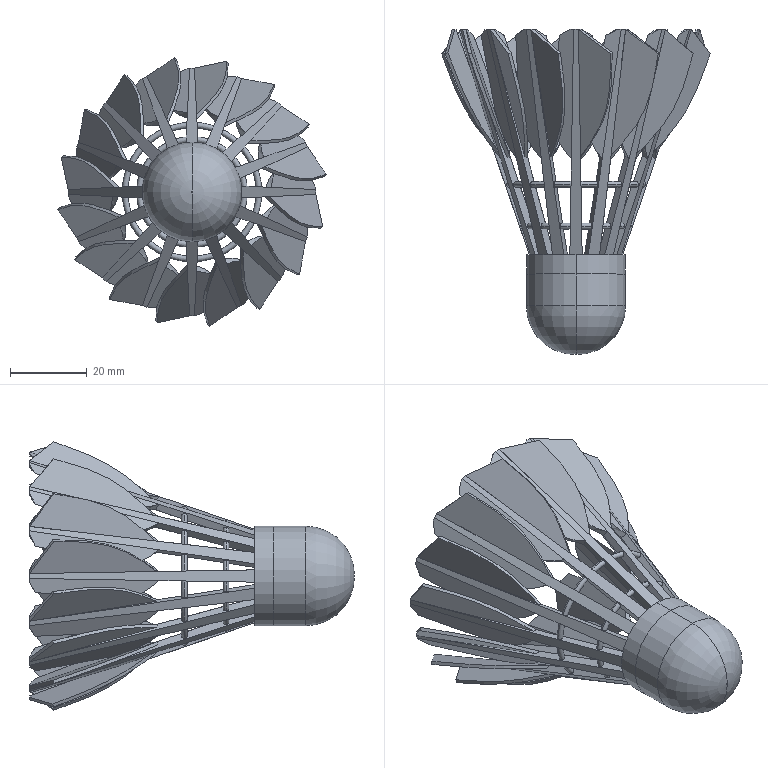Part | SolidWorks | features CirPattern 3, ICE 3, CombineBodies 2, Revolution 2, Blend 1, PLine 1 | 1 solid | 280 faces | box 70.034 x 84.754 x 70.034 mm | volume 20525 mm3 | plane 178 | torus 66 | cylinder 20 | spline 16 | commonest cylinder face diameters 29.581 x16 26 x4